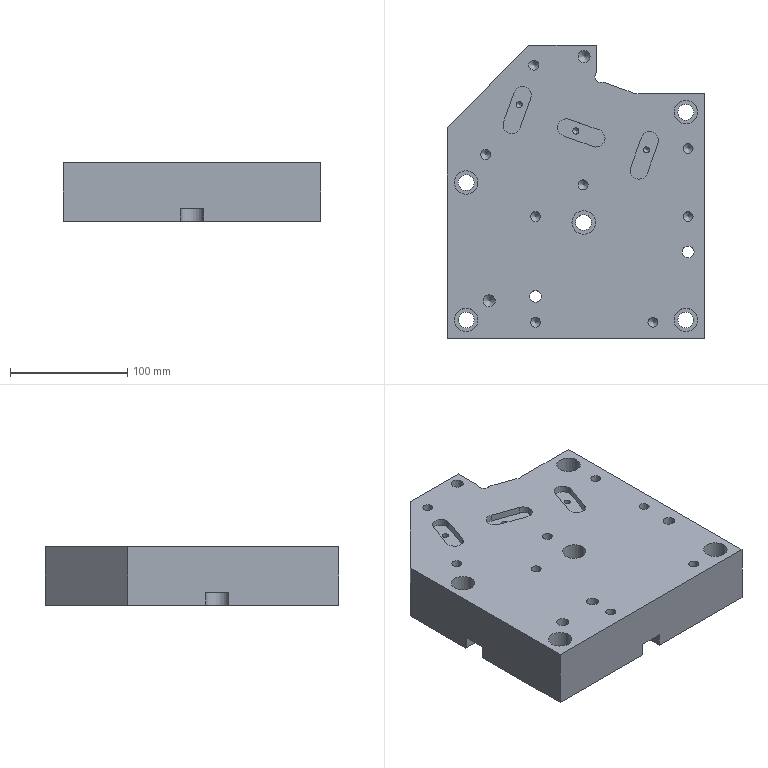Part | NX | features solid 2 | 1 solid | 90 faces | box 219 x 250 x 50 mm | volume 2299023 mm3 | cylinder 42 | plane 35 | cone 13 | commonest cylinder face diameters 20 x12 8.5 x8 15 x6 13.5 x5 5.2 x3 10 x2